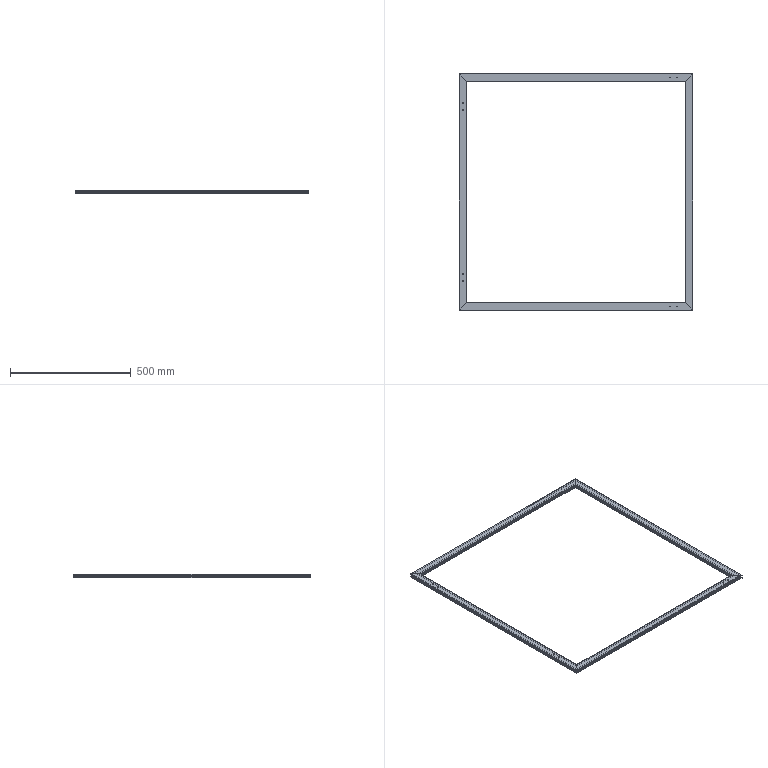Part | SolidWorks | features WeldCornerFeat 4, HoleWzd 2, 3DProfileFeature 1, WeldMemberFeat 1, WeldmentFeature 1 | 4 solids | 176 faces | box 967 x 978 x 15 mm | volume 980488 mm3 | plane 120 | cylinder 48 | cone 8 | commonest cylinder face diameters 5 x32 3.3 x16